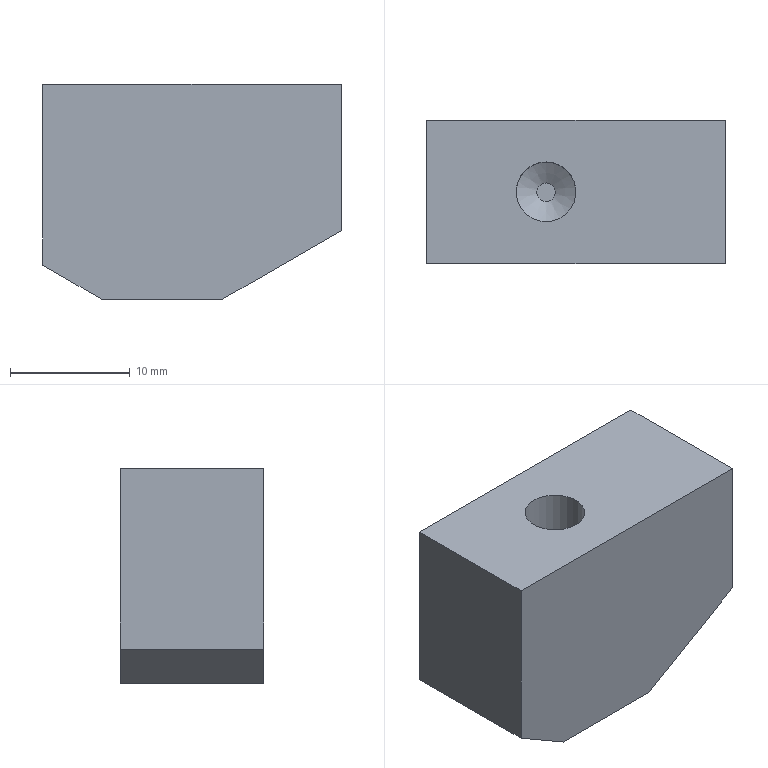Part | STEP file | solid 125 | 1 solid | 11 faces | box 25 x 12 x 18 mm | volume 4663 mm3 | plane 9 | cylinder 1 | cone 1 | commonest cylinder face diameters 5 x1